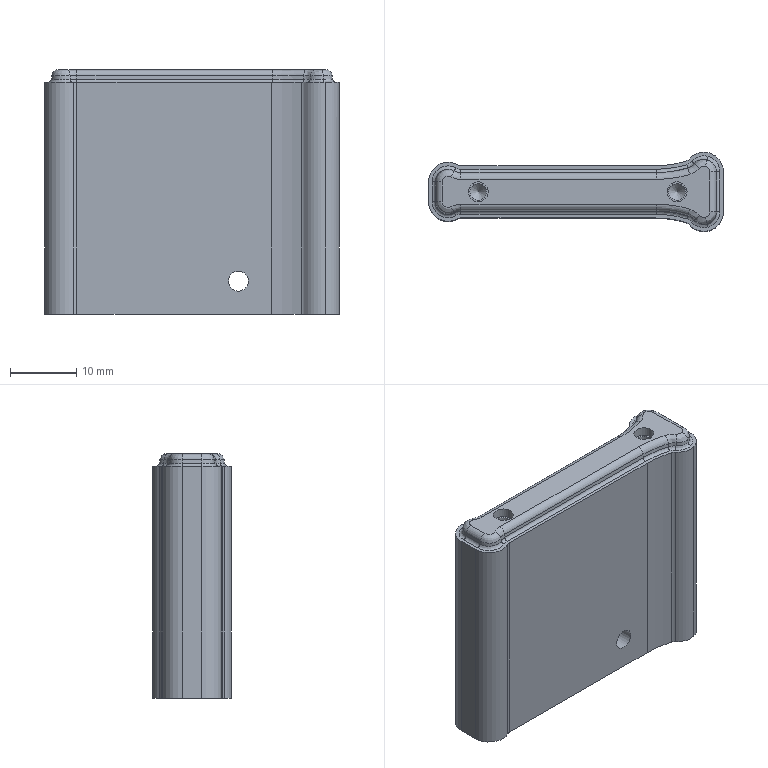Part | NX | features DIE-97 2 | 1 solid | 76 faces | box 44.498 x 11.926 x 36.9 mm | volume 13276 mm3 | spline 24 | cylinder 19 | plane 13 | torus 12 | cone 8 | commonest cylinder face diameters 1 x4 2 x4 3 x3 2.1 x2 2.506 x2 5.9 x2